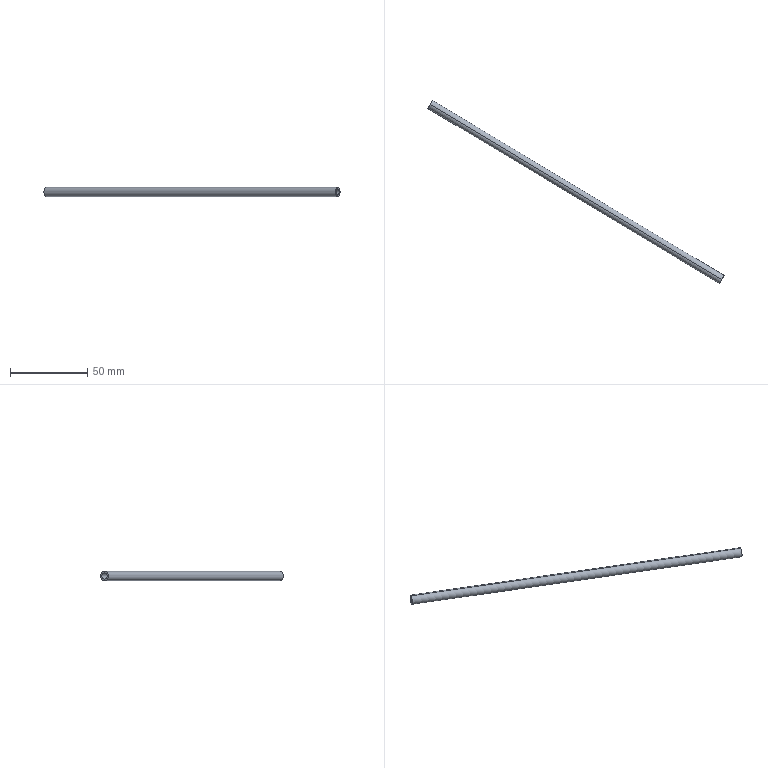Part | SolidWorks | features BaseBody 1 | 1 solid | 6 faces | box 191.667 x 118.451 x 6 mm | volume 3456 mm3 | cylinder 4 | plane 2 | commonest cylinder face diameters 4 x2 6 x2
STEP:
#1=CARTESIAN_POINT('',(-179.153,181.661,-249.5));
#2=VERTEX_POINT('',#1);
#3=CARTESIAN_POINT('',(-179.153,181.661,-245.5));
#4=VERTEX_POINT('',#3);
#5=CARTESIAN_POINT('',(-179.153,181.661,-247.5));
#6=DIRECTION('',(-0.8572,0.515,0.));
#7=DIRECTION('',(-0.515,-0.8572,0.));
#8=AXIS2_PLACEMENT_3D('',#5,#6,#7);
#9=CIRCLE('',#8,2.);
#10=EDGE_CURVE('',#2,#4,#9,.T.);
#11=ORIENTED_EDGE('',*,*,#10,.T.);
#12=CARTESIAN_POINT('',(9.424,68.353,-245.5));
#13=VERTEX_POINT('',#12);
#14=CARTESIAN_POINT('',(9.424,68.353,-245.5));
#15=DIRECTION('',(0.8572,-0.515,0.));
#16=VECTOR('',#15,1000.);
#17=LINE('',#14,#16);
#18=EDGE_CURVE('',#4,#13,#17,.T.);
#19=ORIENTED_EDGE('',*,*,#18,.T.);
#20=CARTESIAN_POINT('',(9.424,68.353,-249.5));
#21=VERTEX_POINT('',#20);
#22=CARTESIAN_POINT('',(9.424,68.353,-247.5));
#23=DIRECTION('',(-0.8572,0.515,0.));
#24=DIRECTION('',(0.,0.,-1.));
#25=AXIS2_PLACEMENT_3D('',#22,#23,#24);
#26=CIRCLE('',#25,2.);
#27=EDGE_CURVE('',#21,#13,#26,.T.);
#28=ORIENTED_EDGE('',*,*,#27,.F.);
#29=CARTESIAN_POINT('',(9.424,68.353,-249.5));
#30=DIRECTION('',(0.8572,-0.515,0.));
#31=VECTOR('',#30,1000.);
#32=LINE('',#29,#31);
#33=EDGE_CURVE('',#2,#21,#32,.T.);
#34=ORIENTED_EDGE('',*,*,#33,.F.);
#35=EDGE_LOOP('',(#11,#19,#28,#34));
#36=FACE_OUTER_BOUND('',#35,.T.);
#37=CARTESIAN_POINT('',(9.424,68.353,-247.5));
#38=DIRECTION('',(0.8572,-0.515,0.));
#39=DIRECTION('',(0.,0.,-1.));
#40=AXIS2_PLACEMENT_3D('',#37,#38,#39);
#41=CYLINDRICAL_SURFACE('',#40,2.);
#42=ADVANCED_FACE('',(#36),#41,.F.);
#43=CARTESIAN_POINT('',(-179.153,181.661,-244.5));
#44=VERTEX_POINT('',#43);
#45=CARTESIAN_POINT('',(-179.153,181.661,-250.5));
#46=VERTEX_POINT('',#45);
#47=CARTESIAN_POINT('',(-179.153,181.661,-247.5));
#48=DIRECTION('',(-0.8572,0.515,0.));
#49=DIRECTION('',(-0.515,-0.8572,0.));
#50=AXIS2_PLACEMENT_3D('',#47,#48,#49);
#51=CIRCLE('',#50,3.);
#52=EDGE_CURVE('',#44,#46,#51,.T.);
#53=ORIENTED_EDGE('',*,*,#52,.F.);
#54=CARTESIAN_POINT('',(9.424,68.353,-244.5));
#55=VERTEX_POINT('',#54);
#56=CARTESIAN_POINT('',(9.424,68.353,-244.5));
#57=DIRECTION('',(0.8572,-0.515,0.));
#58=VECTOR('',#57,1000.);
#59=LINE('',#56,#58);
#60=EDGE_CURVE('',#44,#55,#59,.T.);
#61=ORIENTED_EDGE('',*,*,#60,.T.);
#62=CARTESIAN_POINT('',(9.424,68.353,-250.5));
#63=VERTEX_POINT('',#62);
#64=CARTESIAN_POINT('',(9.424,68.353,-247.5));
#65=DIRECTION('',(-0.8572,0.515,0.));
#66=DIRECTION('',(0.,0.,-1.));
#67=AXIS2_PLACEMENT_3D('',#64,#65,#66);
#68=CIRCLE('',#67,3.);
#69=EDGE_CURVE('',#55,#63,#68,.T.);
#70=ORIENTED_EDGE('',*,*,#69,.T.);
#71=CARTESIAN_POINT('',(9.424,68.353,-250.5));
#72=DIRECTION('',(0.8572,-0.515,0.));
#73=VECTOR('',#72,1000.);
#74=LINE('',#71,#73);
#75=EDGE_CURVE('',#46,#63,#74,.T.);
#76=ORIENTED_EDGE('',*,*,#75,.F.);
#77=EDGE_LOOP('',(#53,#61,#70,#76));
#78=FACE_OUTER_BOUND('',#77,.T.);
#79=CARTESIAN_POINT('',(9.424,68.353,-247.5));
#80=DIRECTION('',(0.8572,-0.515,0.));
#81=DIRECTION('',(0.,0.,-1.));
#82=AXIS2_PLACEMENT_3D('',#79,#80,#81);
#83=CYLINDRICAL_SURFACE('',#82,3.);
#84=ADVANCED_FACE('',(#78),#83,.T.);
#85=ORIENTED_EDGE('',*,*,#60,.F.);
#86=CARTESIAN_POINT('',(-179.153,181.661,-247.5));
#87=DIRECTION('',(-0.8572,0.515,0.));
#88=DIRECTION('',(-0.515,-0.8572,0.));
#89=AXIS2_PLACEMENT_3D('',#86,#87,#88);
#90=CIRCLE('',#89,3.);
#91=EDGE_CURVE('',#46,#44,#90,.T.);
#92=ORIENTED_EDGE('',*,*,#91,.F.);
#93=ORIENTED_EDGE('',*,*,#75,.T.);
#94=CARTESIAN_POINT('',(9.424,68.353,-247.5));
#95=DIRECTION('',(-0.8572,0.515,0.));
#96=DIRECTION('',(0.,0.,-1.));
#97=AXIS2_PLACEMENT_3D('',#94,#95,#96);
#98=CIRCLE('',#97,3.);
#99=EDGE_CURVE('',#63,#55,#98,.T.);
#100=ORIENTED_EDGE('',*,*,#99,.T.);
#101=EDGE_LOOP('',(#85,#92,#93,#100));
#102=FACE_OUTER_BOUND('',#101,.T.);
#103=CARTESIAN_POINT('',(9.424,68.353,-247.5));
#104=DIRECTION('',(0.8572,-0.515,0.));
#105=DIRECTION('',(0.,0.,-1.));
#106=AXIS2_PLACEMENT_3D('',#103,#104,#105);
#107=CYLINDRICAL_SURFACE('',#106,3.);
#108=ADVANCED_FACE('',(#102),#107,.T.);
#109=ORIENTED_EDGE('',*,*,#10,.F.);
#110=CARTESIAN_POINT('',(-179.153,181.661,-247.5));
#111=DIRECTION('',(-0.8572,0.515,0.));
#112=DIRECTION('',(-0.515,-0.8572,0.));
#113=AXIS2_PLACEMENT_3D('',#110,#111,#112);
#114=CIRCLE('',#113,2.);
#115=EDGE_CURVE('',#4,#2,#114,.T.);
#116=ORIENTED_EDGE('',*,*,#115,.F.);
#117=EDGE_LOOP('',(#109,#116));
#118=FACE_BOUND('',#117,.T.);
#119=ORIENTED_EDGE('',*,*,#91,.T.);
#120=ORIENTED_EDGE('',*,*,#52,.T.);
#121=EDGE_LOOP('',(#119,#120));
#122=FACE_OUTER_BOUND('',#121,.T.);
#123=CARTESIAN_POINT('',(-180.698,179.09,-247.5));
#124=DIRECTION('',(-0.8572,0.515,0.));
#125=DIRECTION('',(0.,0.,1.));
#126=AXIS2_PLACEMENT_3D('',#123,#124,#125);
#127=PLANE('',#126);
#128=ADVANCED_FACE('',(#118,#122),#127,.T.);
#129=ORIENTED_EDGE('',*,*,#18,.F.);
#130=ORIENTED_EDGE('',*,*,#115,.T.);
#131=ORIENTED_EDGE('',*,*,#33,.T.);
#132=CARTESIAN_POINT('',(9.424,68.353,-247.5));
#133=DIRECTION('',(-0.8572,0.515,0.));
#134=DIRECTION('',(0.,0.,-1.));
#135=AXIS2_PLACEMENT_3D('',#132,#133,#134);
#136=CIRCLE('',#135,2.);
#137=EDGE_CURVE('',#13,#21,#136,.T.);
#138=ORIENTED_EDGE('',*,*,#137,.F.);
#139=EDGE_LOOP('',(#129,#130,#131,#138));
#140=FACE_OUTER_BOUND('',#139,.T.);
#141=CARTESIAN_POINT('',(9.424,68.353,-247.5));
#142=DIRECTION('',(0.8572,-0.515,0.));
#143=DIRECTION('',(0.,0.,-1.));
#144=AXIS2_PLACEMENT_3D('',#141,#142,#143);
#145=CYLINDRICAL_SURFACE('',#144,2.);
#146=ADVANCED_FACE('',(#140),#145,.F.);
#147=ORIENTED_EDGE('',*,*,#99,.F.);
#148=ORIENTED_EDGE('',*,*,#69,.F.);
#149=EDGE_LOOP('',(#147,#148));
#150=FACE_OUTER_BOUND('',#149,.T.);
#151=ORIENTED_EDGE('',*,*,#27,.T.);
#152=ORIENTED_EDGE('',*,*,#137,.T.);
#153=EDGE_LOOP('',(#151,#152));
#154=FACE_BOUND('',#153,.T.);
#155=CARTESIAN_POINT('',(8.394,66.638,-247.5));
#156=DIRECTION('',(0.8572,-0.515,0.));
#157=DIRECTION('',(0.,0.,-1.));
#158=AXIS2_PLACEMENT_3D('',#155,#156,#157);
#159=PLANE('',#158);
#160=ADVANCED_FACE('',(#150,#154),#159,.T.);
#161=CLOSED_SHELL('',(#42,#84,#108,#128,#146,#160));
#162=MANIFOLD_SOLID_BREP('',#161);
#163=CARTESIAN_POINT('',(0.,0.,0.));
#164=DIRECTION('',(0.,0.,1.));
#165=DIRECTION('',(1.,0.,0.));
#166=AXIS2_PLACEMENT_3D('',#163,#164,#165);
#167=(LENGTH_UNIT()NAMED_UNIT(*)SI_UNIT(.MILLI.,.METRE.));
#168=UNCERTAINTY_MEASURE_WITH_UNIT(LENGTH_MEASURE(0.00001),#167,'','');
#169=(NAMED_UNIT(*)PLANE_ANGLE_UNIT()SI_UNIT($,.RADIAN.));
#170=(NAMED_UNIT(*)SI_UNIT($,.STERADIAN.)SOLID_ANGLE_UNIT());
#171=(GEOMETRIC_REPRESENTATION_CONTEXT(3)GLOBAL_UNCERTAINTY_ASSIGNED_CONTEXT((#168))GLOBAL_UNIT_ASSIGNED_CONTEXT((#167,#169,#170))REPRESENTATION_CONTEXT('',''));
#172=ADVANCED_BREP_SHAPE_REPRESENTATION('',(#162,#166),#171);